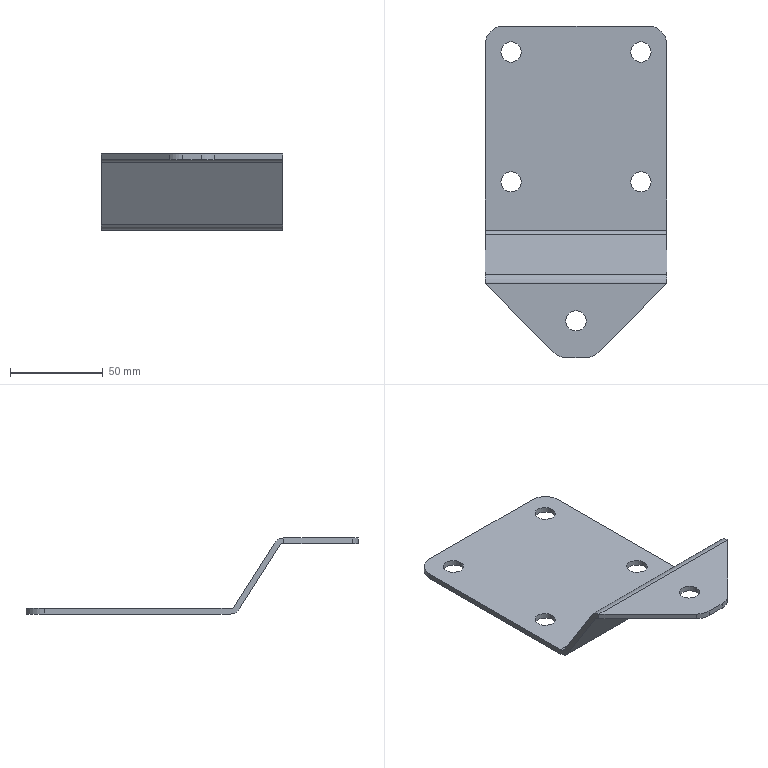Part | STEP file | torque arm 110 | 1 solid | 25 faces | box 98 x 179 x 41 mm | volume 52160 mm3 | plane 12 | cylinder 8 | spline 5 | commonest cylinder face diameters 20 x4 6 x2 12 x2